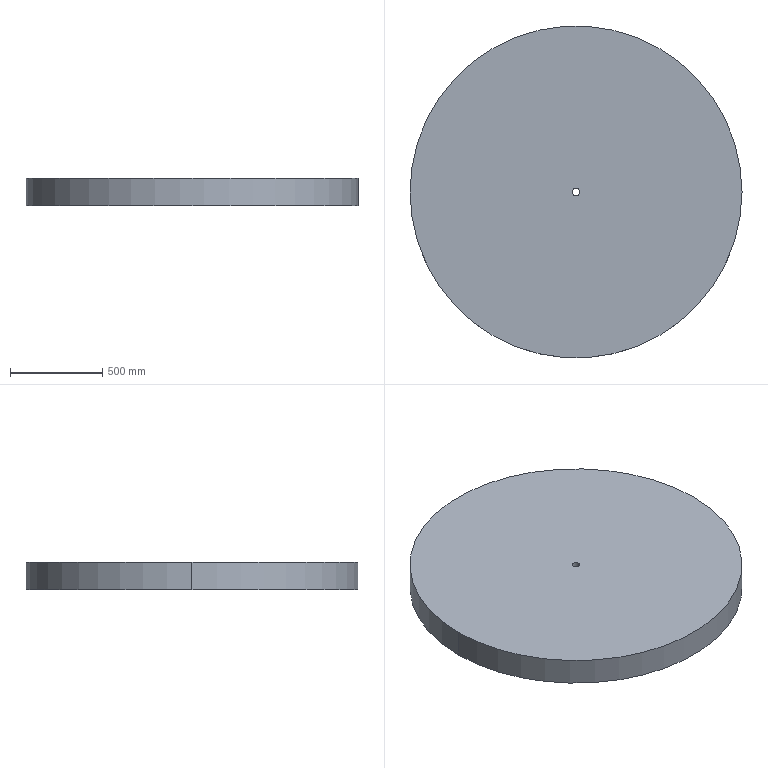Part | SolidWorks | features Extrusion 1, ICE 1 | 1 solid | 6 faces | box 1800 x 1800 x 150 mm | volume 381515012 mm3 | cylinder 4 | plane 2 | commonest cylinder face diameters 40 x2 1800 x2
STEP:
#1=CARTESIAN_POINT('',(20.,0.,150.));
#2=VERTEX_POINT('',#1);
#3=CARTESIAN_POINT('',(-20.,0.,150.));
#4=VERTEX_POINT('',#3);
#5=CARTESIAN_POINT('',(0.,0.,150.));
#6=DIRECTION('',(0.,0.,-1.));
#7=DIRECTION('',(-1.,0.,0.));
#8=AXIS2_PLACEMENT_3D('',#5,#6,#7);
#9=CIRCLE('',#8,20.);
#10=EDGE_CURVE('',#2,#4,#9,.T.);
#11=ORIENTED_EDGE('',*,*,#10,.F.);
#12=CARTESIAN_POINT('',(20.,0.,0.));
#13=VERTEX_POINT('',#12);
#14=CARTESIAN_POINT('',(20.,0.,150.));
#15=DIRECTION('',(0.,0.,-1.));
#16=VECTOR('',#15,1000.);
#17=LINE('',#14,#16);
#18=EDGE_CURVE('',#2,#13,#17,.T.);
#19=ORIENTED_EDGE('',*,*,#18,.T.);
#20=CARTESIAN_POINT('',(-20.,0.,0.));
#21=VERTEX_POINT('',#20);
#22=CARTESIAN_POINT('',(0.,0.,0.));
#23=DIRECTION('',(0.,0.,-1.));
#24=DIRECTION('',(-1.,0.,0.));
#25=AXIS2_PLACEMENT_3D('',#22,#23,#24);
#26=CIRCLE('',#25,20.);
#27=EDGE_CURVE('',#13,#21,#26,.T.);
#28=ORIENTED_EDGE('',*,*,#27,.T.);
#29=CARTESIAN_POINT('',(-20.,0.,150.));
#30=DIRECTION('',(0.,0.,-1.));
#31=VECTOR('',#30,1000.);
#32=LINE('',#29,#31);
#33=EDGE_CURVE('',#4,#21,#32,.T.);
#34=ORIENTED_EDGE('',*,*,#33,.F.);
#35=EDGE_LOOP('',(#11,#19,#28,#34));
#36=FACE_OUTER_BOUND('',#35,.T.);
#37=CARTESIAN_POINT('',(0.,0.,150.));
#38=DIRECTION('',(0.,0.,-1.));
#39=DIRECTION('',(-1.,0.,0.));
#40=AXIS2_PLACEMENT_3D('',#37,#38,#39);
#41=CYLINDRICAL_SURFACE('',#40,20.);
#42=ADVANCED_FACE('',(#36),#41,.F.);
#43=CARTESIAN_POINT('',(900.,0.,150.));
#44=VERTEX_POINT('',#43);
#45=CARTESIAN_POINT('',(-900.,0.,150.));
#46=VERTEX_POINT('',#45);
#47=CARTESIAN_POINT('',(0.,0.,150.));
#48=DIRECTION('',(0.,0.,1.));
#49=DIRECTION('',(1.,0.,0.));
#50=AXIS2_PLACEMENT_3D('',#47,#48,#49);
#51=CIRCLE('',#50,900.);
#52=EDGE_CURVE('',#44,#46,#51,.T.);
#53=ORIENTED_EDGE('',*,*,#52,.F.);
#54=CARTESIAN_POINT('',(900.,0.,0.));
#55=VERTEX_POINT('',#54);
#56=CARTESIAN_POINT('',(900.,0.,150.));
#57=DIRECTION('',(0.,0.,-1.));
#58=VECTOR('',#57,1000.);
#59=LINE('',#56,#58);
#60=EDGE_CURVE('',#44,#55,#59,.T.);
#61=ORIENTED_EDGE('',*,*,#60,.T.);
#62=CARTESIAN_POINT('',(-900.,0.,0.));
#63=VERTEX_POINT('',#62);
#64=CARTESIAN_POINT('',(0.,0.,0.));
#65=DIRECTION('',(0.,0.,1.));
#66=DIRECTION('',(1.,0.,0.));
#67=AXIS2_PLACEMENT_3D('',#64,#65,#66);
#68=CIRCLE('',#67,900.);
#69=EDGE_CURVE('',#55,#63,#68,.T.);
#70=ORIENTED_EDGE('',*,*,#69,.T.);
#71=CARTESIAN_POINT('',(-900.,0.,150.));
#72=DIRECTION('',(0.,0.,-1.));
#73=VECTOR('',#72,1000.);
#74=LINE('',#71,#73);
#75=EDGE_CURVE('',#46,#63,#74,.T.);
#76=ORIENTED_EDGE('',*,*,#75,.F.);
#77=EDGE_LOOP('',(#53,#61,#70,#76));
#78=FACE_OUTER_BOUND('',#77,.T.);
#79=CARTESIAN_POINT('',(0.,0.,150.));
#80=DIRECTION('',(0.,0.,-1.));
#81=DIRECTION('',(-1.,0.,0.));
#82=AXIS2_PLACEMENT_3D('',#79,#80,#81);
#83=CYLINDRICAL_SURFACE('',#82,900.);
#84=ADVANCED_FACE('',(#78),#83,.T.);
#85=ORIENTED_EDGE('',*,*,#60,.F.);
#86=CARTESIAN_POINT('',(0.,0.,150.));
#87=DIRECTION('',(0.,0.,1.));
#88=DIRECTION('',(1.,0.,0.));
#89=AXIS2_PLACEMENT_3D('',#86,#87,#88);
#90=CIRCLE('',#89,900.);
#91=EDGE_CURVE('',#46,#44,#90,.T.);
#92=ORIENTED_EDGE('',*,*,#91,.F.);
#93=ORIENTED_EDGE('',*,*,#75,.T.);
#94=CARTESIAN_POINT('',(0.,0.,0.));
#95=DIRECTION('',(0.,0.,1.));
#96=DIRECTION('',(1.,0.,0.));
#97=AXIS2_PLACEMENT_3D('',#94,#95,#96);
#98=CIRCLE('',#97,900.);
#99=EDGE_CURVE('',#63,#55,#98,.T.);
#100=ORIENTED_EDGE('',*,*,#99,.T.);
#101=EDGE_LOOP('',(#85,#92,#93,#100));
#102=FACE_OUTER_BOUND('',#101,.T.);
#103=CARTESIAN_POINT('',(0.,0.,150.));
#104=DIRECTION('',(0.,0.,-1.));
#105=DIRECTION('',(-1.,0.,0.));
#106=AXIS2_PLACEMENT_3D('',#103,#104,#105);
#107=CYLINDRICAL_SURFACE('',#106,900.);
#108=ADVANCED_FACE('',(#102),#107,.T.);
#109=CARTESIAN_POINT('',(0.,0.,150.));
#110=DIRECTION('',(0.,0.,-1.));
#111=DIRECTION('',(-1.,0.,0.));
#112=AXIS2_PLACEMENT_3D('',#109,#110,#111);
#113=CIRCLE('',#112,20.);
#114=EDGE_CURVE('',#4,#2,#113,.T.);
#115=ORIENTED_EDGE('',*,*,#114,.T.);
#116=ORIENTED_EDGE('',*,*,#10,.T.);
#117=EDGE_LOOP('',(#115,#116));
#118=FACE_BOUND('',#117,.T.);
#119=ORIENTED_EDGE('',*,*,#91,.T.);
#120=ORIENTED_EDGE('',*,*,#52,.T.);
#121=EDGE_LOOP('',(#119,#120));
#122=FACE_OUTER_BOUND('',#121,.T.);
#123=CARTESIAN_POINT('',(0.,0.,150.));
#124=DIRECTION('',(0.,0.,1.));
#125=DIRECTION('',(1.,0.,0.));
#126=AXIS2_PLACEMENT_3D('',#123,#124,#125);
#127=PLANE('',#126);
#128=ADVANCED_FACE('',(#118,#122),#127,.T.);
#129=CARTESIAN_POINT('',(0.,0.,0.));
#130=DIRECTION('',(0.,0.,-1.));
#131=DIRECTION('',(-1.,0.,0.));
#132=AXIS2_PLACEMENT_3D('',#129,#130,#131);
#133=CIRCLE('',#132,20.);
#134=EDGE_CURVE('',#21,#13,#133,.T.);
#135=ORIENTED_EDGE('',*,*,#134,.F.);
#136=ORIENTED_EDGE('',*,*,#27,.F.);
#137=EDGE_LOOP('',(#135,#136));
#138=FACE_BOUND('',#137,.T.);
#139=ORIENTED_EDGE('',*,*,#99,.F.);
#140=ORIENTED_EDGE('',*,*,#69,.F.);
#141=EDGE_LOOP('',(#139,#140));
#142=FACE_OUTER_BOUND('',#141,.T.);
#143=CARTESIAN_POINT('',(0.,0.,0.));
#144=DIRECTION('',(0.,0.,1.));
#145=DIRECTION('',(1.,0.,0.));
#146=AXIS2_PLACEMENT_3D('',#143,#144,#145);
#147=PLANE('',#146);
#148=ADVANCED_FACE('',(#138,#142),#147,.F.);
#149=ORIENTED_EDGE('',*,*,#18,.F.);
#150=ORIENTED_EDGE('',*,*,#114,.F.);
#151=ORIENTED_EDGE('',*,*,#33,.T.);
#152=ORIENTED_EDGE('',*,*,#134,.T.);
#153=EDGE_LOOP('',(#149,#150,#151,#152));
#154=FACE_OUTER_BOUND('',#153,.T.);
#155=CARTESIAN_POINT('',(0.,0.,150.));
#156=DIRECTION('',(0.,0.,-1.));
#157=DIRECTION('',(-1.,0.,0.));
#158=AXIS2_PLACEMENT_3D('',#155,#156,#157);
#159=CYLINDRICAL_SURFACE('',#158,20.);
#160=ADVANCED_FACE('',(#154),#159,.F.);
#161=CLOSED_SHELL('',(#42,#84,#108,#128,#148,#160));
#162=MANIFOLD_SOLID_BREP('',#161);
#163=CARTESIAN_POINT('',(0.,0.,0.));
#164=DIRECTION('',(0.,0.,1.));
#165=DIRECTION('',(1.,0.,0.));
#166=AXIS2_PLACEMENT_3D('',#163,#164,#165);
#167=(LENGTH_UNIT()NAMED_UNIT(*)SI_UNIT(.MILLI.,.METRE.));
#168=UNCERTAINTY_MEASURE_WITH_UNIT(LENGTH_MEASURE(0.00001),#167,'','');
#169=(NAMED_UNIT(*)PLANE_ANGLE_UNIT()SI_UNIT($,.RADIAN.));
#170=(NAMED_UNIT(*)SI_UNIT($,.STERADIAN.)SOLID_ANGLE_UNIT());
#171=(GEOMETRIC_REPRESENTATION_CONTEXT(3)GLOBAL_UNCERTAINTY_ASSIGNED_CONTEXT((#168))GLOBAL_UNIT_ASSIGNED_CONTEXT((#167,#169,#170))REPRESENTATION_CONTEXT('',''));
#172=ADVANCED_BREP_SHAPE_REPRESENTATION('',(#162,#166),#171);